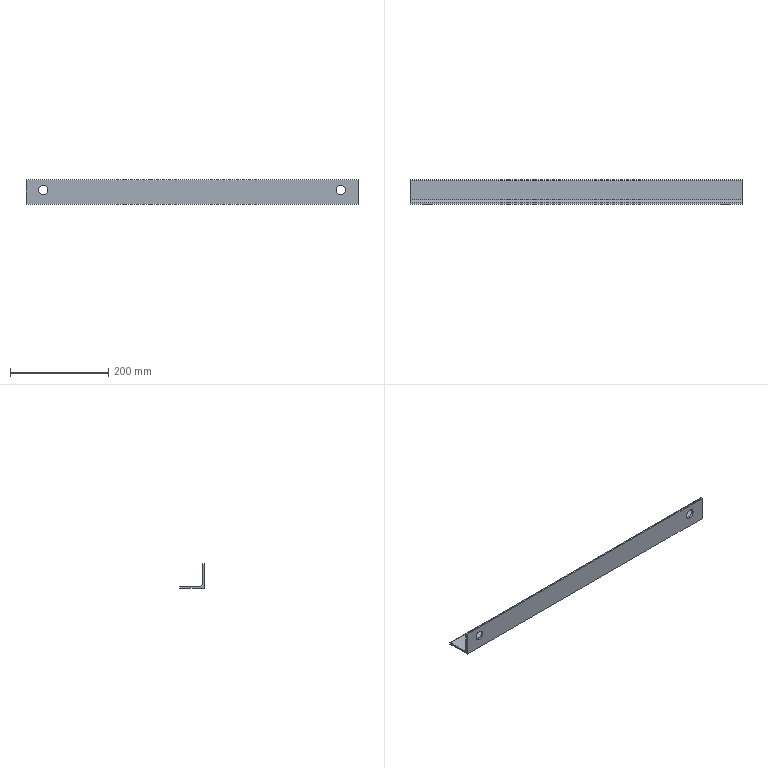Part | STEP file | 电柜角钢2_Default<As Machined> | 1 solid | 15 faces | box 675 x 50 x 50 mm | volume 260801 mm3 | plane 8 | cylinder 7 | commonest cylinder face diameters 19 x4 2.66 x2 11 x1
STEP:
#1=CARTESIAN_POINT('',(0.,0.,0.));
#2=DIRECTION('',(0.,0.,1.));
#3=DIRECTION('',(1.,0.,0.));
#4=AXIS2_PLACEMENT_3D('',#1,#2,#3);
#5=CARTESIAN_POINT('',(-302.5,0.,38.585));
#6=VERTEX_POINT('',#5);
#7=CARTESIAN_POINT('',(-302.5,4.,38.585));
#8=VERTEX_POINT('',#7);
#9=CARTESIAN_POINT('',(-302.5,-6.,38.585));
#10=DIRECTION('',(0.,1.,0.));
#11=VECTOR('',#10,1.);
#12=LINE('',#9,#11);
#13=CARTESIAN_POINT('',(-302.5,-6.,29.085));
#14=DIRECTION('',(0.,1.,0.));
#15=DIRECTION('',(0.,0.,1.));
#16=AXIS2_PLACEMENT_3D('',#13,#14,#15);
#17=CYLINDRICAL_SURFACE('',#16,9.5);
#18=CARTESIAN_POINT('',(6.283,0.));
#19=DIRECTION('',(0.,1.));
#20=VECTOR('',#19,1.);
#21=LINE('',#18,#20);
#22=(GEOMETRIC_REPRESENTATION_CONTEXT(2)PARAMETRIC_REPRESENTATION_CONTEXT()REPRESENTATION_CONTEXT('',''));
#23=DEFINITIONAL_REPRESENTATION('',(#21),#22);
#24=PCURVE('',#17,#23);
#25=CARTESIAN_POINT('',(-302.5,-6.,29.085));
#26=DIRECTION('',(0.,1.,0.));
#27=DIRECTION('',(0.,0.,1.));
#28=AXIS2_PLACEMENT_3D('',#25,#26,#27);
#29=CYLINDRICAL_SURFACE('',#28,9.5);
#30=CARTESIAN_POINT('',(0.,0.));
#31=DIRECTION('',(0.,1.));
#32=VECTOR('',#31,1.);
#33=LINE('',#30,#32);
#34=(GEOMETRIC_REPRESENTATION_CONTEXT(2)PARAMETRIC_REPRESENTATION_CONTEXT()REPRESENTATION_CONTEXT('',''));
#35=DEFINITIONAL_REPRESENTATION('',(#33),#34);
#36=PCURVE('',#29,#35);
#37=SURFACE_CURVE('',#12,(#24,#36),.PCURVE_S1.);
#38=EDGE_CURVE('',#6,#8,#37,.T.);
#39=ORIENTED_EDGE('',*,*,#38,.T.);
#40=CARTESIAN_POINT('',(-302.5,4.,19.585));
#41=VERTEX_POINT('',#40);
#42=CARTESIAN_POINT('',(-302.5,4.,29.085));
#43=DIRECTION('',(0.,1.,0.));
#44=DIRECTION('',(0.,0.,1.));
#45=AXIS2_PLACEMENT_3D('',#42,#43,#44);
#46=CIRCLE('',#45,9.5);
#47=CARTESIAN_POINT('',(0.,10.));
#48=DIRECTION('',(1.,0.));
#49=VECTOR('',#48,1.);
#50=LINE('',#47,#49);
#51=(GEOMETRIC_REPRESENTATION_CONTEXT(2)PARAMETRIC_REPRESENTATION_CONTEXT()REPRESENTATION_CONTEXT('',''));
#52=DEFINITIONAL_REPRESENTATION('',(#50),#51);
#53=PCURVE('',#17,#52);
#54=CARTESIAN_POINT('',(337.5,4.,48.67));
#55=DIRECTION('',(0.,-1.,0.));
#56=DIRECTION('',(1.,0.,0.));
#57=AXIS2_PLACEMENT_3D('',#54,#55,#56);
#58=PLANE('',#57);
#59=CARTESIAN_POINT('',(-640.,-10.085));
#60=CARTESIAN_POINT('',(-623.546,-10.085));
#61=CARTESIAN_POINT('',(-631.773,-24.335));
#62=CARTESIAN_POINT('',(-640.,-38.585));
#63=CARTESIAN_POINT('',(-648.227,-24.335));
#64=CARTESIAN_POINT('',(-656.454,-10.085));
#65=CARTESIAN_POINT('',(-640.,-10.085));
#66=(BOUNDED_CURVE()B_SPLINE_CURVE(2,(#59,#60,#61,#62,#63,#64,#65),.UNSPECIFIED.,.T.,.F.)B_SPLINE_CURVE_WITH_KNOTS((1,2,2,2,2,1),(-2.094,0.,2.094,4.189,6.283,8.378),.UNSPECIFIED.)CURVE()GEOMETRIC_REPRESENTATION_ITEM()RATIONAL_B_SPLINE_CURVE((1.,0.5,1.,0.5,1.,0.5,1.))REPRESENTATION_ITEM(''));
#67=(GEOMETRIC_REPRESENTATION_CONTEXT(2)PARAMETRIC_REPRESENTATION_CONTEXT()REPRESENTATION_CONTEXT('',''));
#68=DEFINITIONAL_REPRESENTATION('',(#66),#67);
#69=PCURVE('',#58,#68);
#70=SURFACE_CURVE('',#46,(#53,#69),.PCURVE_S1.);
#71=EDGE_CURVE('',#41,#8,#70,.T.);
#72=ORIENTED_EDGE('',*,*,#71,.F.);
#73=CARTESIAN_POINT('',(-302.5,0.,19.585));
#74=VERTEX_POINT('',#73);
#75=CARTESIAN_POINT('',(-302.5,-6.,19.585));
#76=DIRECTION('',(0.,1.,0.));
#77=VECTOR('',#76,1.);
#78=LINE('',#75,#77);
#79=CARTESIAN_POINT('',(3.142,0.));
#80=DIRECTION('',(0.,1.));
#81=VECTOR('',#80,1.);
#82=LINE('',#79,#81);
#83=(GEOMETRIC_REPRESENTATION_CONTEXT(2)PARAMETRIC_REPRESENTATION_CONTEXT()REPRESENTATION_CONTEXT('',''));
#84=DEFINITIONAL_REPRESENTATION('',(#82),#83);
#85=PCURVE('',#17,#84);
#86=CARTESIAN_POINT('',(3.142,0.));
#87=DIRECTION('',(0.,1.));
#88=VECTOR('',#87,1.);
#89=LINE('',#86,#88);
#90=(GEOMETRIC_REPRESENTATION_CONTEXT(2)PARAMETRIC_REPRESENTATION_CONTEXT()REPRESENTATION_CONTEXT('',''));
#91=DEFINITIONAL_REPRESENTATION('',(#89),#90);
#92=PCURVE('',#29,#91);
#93=SURFACE_CURVE('',#78,(#85,#92),.PCURVE_S1.);
#94=EDGE_CURVE('',#74,#41,#93,.T.);
#95=ORIENTED_EDGE('',*,*,#94,.F.);
#96=CARTESIAN_POINT('',(-302.5,0.,29.085));
#97=DIRECTION('',(0.,1.,0.));
#98=DIRECTION('',(-1.,0.,0.));
#99=AXIS2_PLACEMENT_3D('',#96,#97,#98);
#100=CIRCLE('',#99,9.5);
#101=CARTESIAN_POINT('',(-1.571,6.));
#102=DIRECTION('',(1.,0.));
#103=VECTOR('',#102,1.);
#104=LINE('',#101,#103);
#105=(GEOMETRIC_REPRESENTATION_CONTEXT(2)PARAMETRIC_REPRESENTATION_CONTEXT()REPRESENTATION_CONTEXT('',''));
#106=DEFINITIONAL_REPRESENTATION('',(#104),#105);
#107=PCURVE('',#17,#106);
#108=CARTESIAN_POINT('',(337.5,0.,50.));
#109=DIRECTION('',(0.,1.,0.));
#110=DIRECTION('',(-1.,0.,0.));
#111=AXIS2_PLACEMENT_3D('',#108,#109,#110);
#112=PLANE('',#111);
#113=CARTESIAN_POINT('',(640.,-20.915));
#114=DIRECTION('',(1.,0.));
#115=AXIS2_PLACEMENT_2D('',#113,#114);
#116=CIRCLE('',#115,9.5);
#117=(GEOMETRIC_REPRESENTATION_CONTEXT(2)PARAMETRIC_REPRESENTATION_CONTEXT()REPRESENTATION_CONTEXT('',''));
#118=DEFINITIONAL_REPRESENTATION('',(#116),#117);
#119=PCURVE('',#112,#118);
#120=SURFACE_CURVE('',#100,(#107,#119),.PCURVE_S1.);
#121=EDGE_CURVE('',#74,#6,#120,.T.);
#122=ORIENTED_EDGE('',*,*,#121,.T.);
#123=EDGE_LOOP('',(#39,#72,#95,#122));
#124=FACE_BOUND('',#123,.F.);
#125=ADVANCED_FACE('',(#124),#17,.F.);
#126=CARTESIAN_POINT('',(302.5,0.,38.585));
#127=VERTEX_POINT('',#126);
#128=CARTESIAN_POINT('',(302.5,4.,38.585));
#129=VERTEX_POINT('',#128);
#130=CARTESIAN_POINT('',(302.5,-6.,38.585));
#131=DIRECTION('',(0.,1.,0.));
#132=VECTOR('',#131,1.);
#133=LINE('',#130,#132);
#134=CARTESIAN_POINT('',(302.5,-6.,29.085));
#135=DIRECTION('',(0.,1.,0.));
#136=DIRECTION('',(0.,0.,1.));
#137=AXIS2_PLACEMENT_3D('',#134,#135,#136);
#138=CYLINDRICAL_SURFACE('',#137,9.5);
#139=CARTESIAN_POINT('',(6.283,0.));
#140=DIRECTION('',(0.,1.));
#141=VECTOR('',#140,1.);
#142=LINE('',#139,#141);
#143=(GEOMETRIC_REPRESENTATION_CONTEXT(2)PARAMETRIC_REPRESENTATION_CONTEXT()REPRESENTATION_CONTEXT('',''));
#144=DEFINITIONAL_REPRESENTATION('',(#142),#143);
#145=PCURVE('',#138,#144);
#146=CARTESIAN_POINT('',(302.5,-6.,29.085));
#147=DIRECTION('',(0.,1.,0.));
#148=DIRECTION('',(0.,0.,1.));
#149=AXIS2_PLACEMENT_3D('',#146,#147,#148);
#150=CYLINDRICAL_SURFACE('',#149,9.5);
#151=CARTESIAN_POINT('',(0.,0.));
#152=DIRECTION('',(0.,1.));
#153=VECTOR('',#152,1.);
#154=LINE('',#151,#153);
#155=(GEOMETRIC_REPRESENTATION_CONTEXT(2)PARAMETRIC_REPRESENTATION_CONTEXT()REPRESENTATION_CONTEXT('',''));
#156=DEFINITIONAL_REPRESENTATION('',(#154),#155);
#157=PCURVE('',#150,#156);
#158=SURFACE_CURVE('',#133,(#145,#157),.PCURVE_S1.);
#159=EDGE_CURVE('',#127,#129,#158,.T.);
#160=ORIENTED_EDGE('',*,*,#159,.T.);
#161=CARTESIAN_POINT('',(302.5,4.,19.585));
#162=VERTEX_POINT('',#161);
#163=CARTESIAN_POINT('',(302.5,4.,29.085));
#164=DIRECTION('',(0.,1.,0.));
#165=DIRECTION('',(0.,0.,-1.));
#166=AXIS2_PLACEMENT_3D('',#163,#164,#165);
#167=CIRCLE('',#166,9.5);
#168=CARTESIAN_POINT('',(3.142,10.));
#169=DIRECTION('',(1.,0.));
#170=VECTOR('',#169,1.);
#171=LINE('',#168,#170);
#172=(GEOMETRIC_REPRESENTATION_CONTEXT(2)PARAMETRIC_REPRESENTATION_CONTEXT()REPRESENTATION_CONTEXT('',''));
#173=DEFINITIONAL_REPRESENTATION('',(#171),#172);
#174=PCURVE('',#138,#173);
#175=CARTESIAN_POINT('',(-35.,-29.085));
#176=CARTESIAN_POINT('',(-51.454,-29.085));
#177=CARTESIAN_POINT('',(-43.227,-14.835));
#178=CARTESIAN_POINT('',(-35.,-0.585));
#179=CARTESIAN_POINT('',(-26.773,-14.835));
#180=CARTESIAN_POINT('',(-18.546,-29.085));
#181=CARTESIAN_POINT('',(-35.,-29.085));
#182=(BOUNDED_CURVE()B_SPLINE_CURVE(2,(#175,#176,#177,#178,#179,#180,#181),.UNSPECIFIED.,.T.,.F.)B_SPLINE_CURVE_WITH_KNOTS((1,2,2,2,2,1),(-2.094,0.,2.094,4.189,6.283,8.378),.UNSPECIFIED.)CURVE()GEOMETRIC_REPRESENTATION_ITEM()RATIONAL_B_SPLINE_CURVE((1.,0.5,1.,0.5,1.,0.5,1.))REPRESENTATION_ITEM(''));
#183=(GEOMETRIC_REPRESENTATION_CONTEXT(2)PARAMETRIC_REPRESENTATION_CONTEXT()REPRESENTATION_CONTEXT('',''));
#184=DEFINITIONAL_REPRESENTATION('',(#182),#183);
#185=PCURVE('',#58,#184);
#186=SURFACE_CURVE('',#167,(#174,#185),.PCURVE_S1.);
#187=EDGE_CURVE('',#162,#129,#186,.T.);
#188=ORIENTED_EDGE('',*,*,#187,.F.);
#189=CARTESIAN_POINT('',(302.5,0.,19.585));
#190=VERTEX_POINT('',#189);
#191=CARTESIAN_POINT('',(302.5,-6.,19.585));
#192=DIRECTION('',(0.,1.,0.));
#193=VECTOR('',#192,1.);
#194=LINE('',#191,#193);
#195=CARTESIAN_POINT('',(3.142,0.));
#196=DIRECTION('',(0.,1.));
#197=VECTOR('',#196,1.);
#198=LINE('',#195,#197);
#199=(GEOMETRIC_REPRESENTATION_CONTEXT(2)PARAMETRIC_REPRESENTATION_CONTEXT()REPRESENTATION_CONTEXT('',''));
#200=DEFINITIONAL_REPRESENTATION('',(#198),#199);
#201=PCURVE('',#138,#200);
#202=CARTESIAN_POINT('',(3.142,0.));
#203=DIRECTION('',(0.,1.));
#204=VECTOR('',#203,1.);
#205=LINE('',#202,#204);
#206=(GEOMETRIC_REPRESENTATION_CONTEXT(2)PARAMETRIC_REPRESENTATION_CONTEXT()REPRESENTATION_CONTEXT('',''));
#207=DEFINITIONAL_REPRESENTATION('',(#205),#206);
#208=PCURVE('',#150,#207);
#209=SURFACE_CURVE('',#194,(#201,#208),.PCURVE_S1.);
#210=EDGE_CURVE('',#190,#162,#209,.T.);
#211=ORIENTED_EDGE('',*,*,#210,.F.);
#212=CARTESIAN_POINT('',(302.5,0.,29.085));
#213=DIRECTION('',(0.,1.,0.));
#214=DIRECTION('',(-1.,0.,0.));
#215=AXIS2_PLACEMENT_3D('',#212,#213,#214);
#216=CIRCLE('',#215,9.5);
#217=CARTESIAN_POINT('',(-1.571,6.));
#218=DIRECTION('',(1.,0.));
#219=VECTOR('',#218,1.);
#220=LINE('',#217,#219);
#221=(GEOMETRIC_REPRESENTATION_CONTEXT(2)PARAMETRIC_REPRESENTATION_CONTEXT()REPRESENTATION_CONTEXT('',''));
#222=DEFINITIONAL_REPRESENTATION('',(#220),#221);
#223=PCURVE('',#138,#222);
#224=CARTESIAN_POINT('',(35.,-20.915));
#225=DIRECTION('',(1.,0.));
#226=AXIS2_PLACEMENT_2D('',#224,#225);
#227=CIRCLE('',#226,9.5);
#228=(GEOMETRIC_REPRESENTATION_CONTEXT(2)PARAMETRIC_REPRESENTATION_CONTEXT()REPRESENTATION_CONTEXT('',''));
#229=DEFINITIONAL_REPRESENTATION('',(#227),#228);
#230=PCURVE('',#112,#229);
#231=SURFACE_CURVE('',#216,(#223,#230),.PCURVE_S1.);
#232=EDGE_CURVE('',#190,#127,#231,.T.);
#233=ORIENTED_EDGE('',*,*,#232,.T.);
#234=EDGE_LOOP('',(#160,#188,#211,#233));
#235=FACE_BOUND('',#234,.F.);
#236=ADVANCED_FACE('',(#235),#138,.F.);
#237=CARTESIAN_POINT('',(-337.5,50.,2.67));
#238=VERTEX_POINT('',#237);
#239=CARTESIAN_POINT('',(-337.5,48.67,4.));
#240=VERTEX_POINT('',#239);
#241=CARTESIAN_POINT('',(-337.5,48.67,2.67));
#242=DIRECTION('',(1.,0.,0.));
#243=DIRECTION('',(0.,1.,0.));
#244=AXIS2_PLACEMENT_3D('',#241,#242,#243);
#245=CIRCLE('',#244,1.33);
#246=CARTESIAN_POINT('',(337.5,48.67,2.67));
#247=DIRECTION('',(-1.,0.,0.));
#248=DIRECTION('',(0.,-1.,0.));
#249=AXIS2_PLACEMENT_3D('',#246,#247,#248);
#250=CYLINDRICAL_SURFACE('',#249,1.33);
#251=CARTESIAN_POINT('',(3.142,675.));
#252=DIRECTION('',(-1.,0.));
#253=VECTOR('',#252,1.);
#254=LINE('',#251,#253);
#255=(GEOMETRIC_REPRESENTATION_CONTEXT(2)PARAMETRIC_REPRESENTATION_CONTEXT()REPRESENTATION_CONTEXT('',''));
#256=DEFINITIONAL_REPRESENTATION('',(#254),#255);
#257=PCURVE('',#250,#256);
#258=CARTESIAN_POINT('',(-337.5,48.67,2.67));
#259=DIRECTION('',(1.,0.,0.));
#260=DIRECTION('',(0.,1.,0.));
#261=AXIS2_PLACEMENT_3D('',#258,#259,#260);
#262=PLANE('',#261);
#263=CARTESIAN_POINT('',(0.,0.));
#264=DIRECTION('',(1.,0.));
#265=AXIS2_PLACEMENT_2D('',#263,#264);
#266=CIRCLE('',#265,1.33);
#267=(GEOMETRIC_REPRESENTATION_CONTEXT(2)PARAMETRIC_REPRESENTATION_CONTEXT()REPRESENTATION_CONTEXT('',''));
#268=DEFINITIONAL_REPRESENTATION('',(#266),#267);
#269=PCURVE('',#262,#268);
#270=SURFACE_CURVE('',#245,(#257,#269),.PCURVE_S1.);
#271=EDGE_CURVE('',#238,#240,#270,.T.);
#272=ORIENTED_EDGE('',*,*,#271,.T.);
#273=CARTESIAN_POINT('',(337.5,48.67,4.));
#274=VERTEX_POINT('',#273);
#275=CARTESIAN_POINT('',(337.5,48.67,4.));
#276=DIRECTION('',(-1.,0.,0.));
#277=VECTOR('',#276,1.);
#278=LINE('',#275,#277);
#279=CARTESIAN_POINT('',(1.571,0.));
#280=DIRECTION('',(0.,1.));
#281=VECTOR('',#280,1.);
#282=LINE('',#279,#281);
#283=(GEOMETRIC_REPRESENTATION_CONTEXT(2)PARAMETRIC_REPRESENTATION_CONTEXT()REPRESENTATION_CONTEXT('',''));
#284=DEFINITIONAL_REPRESENTATION('',(#282),#283);
#285=PCURVE('',#250,#284);
#286=CARTESIAN_POINT('',(337.5,9.5,4.));
#287=DIRECTION('',(0.,0.,-1.));
#288=DIRECTION('',(-1.,0.,0.));
#289=AXIS2_PLACEMENT_3D('',#286,#287,#288);
#290=PLANE('',#289);
#291=CARTESIAN_POINT('',(0.,39.17));
#292=DIRECTION('',(1.,0.));
#293=VECTOR('',#292,1.);
#294=LINE('',#291,#293);
#295=(GEOMETRIC_REPRESENTATION_CONTEXT(2)PARAMETRIC_REPRESENTATION_CONTEXT()REPRESENTATION_CONTEXT('',''));
#296=DEFINITIONAL_REPRESENTATION('',(#294),#295);
#297=PCURVE('',#290,#296);
#298=SURFACE_CURVE('',#278,(#285,#297),.PCURVE_S1.);
#299=EDGE_CURVE('',#274,#240,#298,.T.);
#300=ORIENTED_EDGE('',*,*,#299,.F.);
#301=CARTESIAN_POINT('',(337.5,50.,2.67));
#302=VERTEX_POINT('',#301);
#303=CARTESIAN_POINT('',(337.5,48.67,2.67));
#304=DIRECTION('',(1.,0.,0.));
#305=DIRECTION('',(0.,1.,0.));
#306=AXIS2_PLACEMENT_3D('',#303,#304,#305);
#307=CIRCLE('',#306,1.33);
#308=CARTESIAN_POINT('',(3.142,0.));
#309=DIRECTION('',(-1.,0.));
#310=VECTOR('',#309,1.);
#311=LINE('',#308,#310);
#312=(GEOMETRIC_REPRESENTATION_CONTEXT(2)PARAMETRIC_REPRESENTATION_CONTEXT()REPRESENTATION_CONTEXT('',''));
#313=DEFINITIONAL_REPRESENTATION('',(#311),#312);
#314=PCURVE('',#250,#313);
#315=CARTESIAN_POINT('',(337.5,48.67,2.67));
#316=DIRECTION('',(1.,0.,0.));
#317=DIRECTION('',(0.,1.,0.));
#318=AXIS2_PLACEMENT_3D('',#315,#316,#317);
#319=PLANE('',#318);
#320=CARTESIAN_POINT('',(0.,0.));
#321=DIRECTION('',(1.,0.));
#322=AXIS2_PLACEMENT_2D('',#320,#321);
#323=CIRCLE('',#322,1.33);
#324=(GEOMETRIC_REPRESENTATION_CONTEXT(2)PARAMETRIC_REPRESENTATION_CONTEXT()REPRESENTATION_CONTEXT('',''));
#325=DEFINITIONAL_REPRESENTATION('',(#323),#324);
#326=PCURVE('',#319,#325);
#327=SURFACE_CURVE('',#307,(#314,#326),.PCURVE_S1.);
#328=EDGE_CURVE('',#302,#274,#327,.T.);
#329=ORIENTED_EDGE('',*,*,#328,.F.);
#330=CARTESIAN_POINT('',(337.5,50.,2.67));
#331=DIRECTION('',(-1.,0.,0.));
#332=VECTOR('',#331,1.);
#333=LINE('',#330,#332);
#334=CARTESIAN_POINT('',(3.142,0.));
#335=DIRECTION('',(0.,1.));
#336=VECTOR('',#335,1.);
#337=LINE('',#334,#336);
#338=(GEOMETRIC_REPRESENTATION_CONTEXT(2)PARAMETRIC_REPRESENTATION_CONTEXT()REPRESENTATION_CONTEXT('',''));
#339=DEFINITIONAL_REPRESENTATION('',(#337),#338);
#340=PCURVE('',#250,#339);
#341=CARTESIAN_POINT('',(337.5,50.,2.67));
#342=DIRECTION('',(0.,-1.,0.));
#343=DIRECTION('',(1.,0.,0.));
#344=AXIS2_PLACEMENT_3D('',#341,#342,#343);
#345=PLANE('',#344);
#346=CARTESIAN_POINT('',(0.,0.));
#347=DIRECTION('',(-1.,0.));
#348=VECTOR('',#347,1.);
#349=LINE('',#346,#348);
#350=(GEOMETRIC_REPRESENTATION_CONTEXT(2)PARAMETRIC_REPRESENTATION_CONTEXT()REPRESENTATION_CONTEXT('',''));
#351=DEFINITIONAL_REPRESENTATION('',(#349),#350);
#352=PCURVE('',#345,#351);
#353=SURFACE_CURVE('',#333,(#340,#352),.PCURVE_S1.);
#354=EDGE_CURVE('',#302,#238,#353,.T.);
#355=ORIENTED_EDGE('',*,*,#354,.T.);
#356=EDGE_LOOP('',(#272,#300,#329,#355));
#357=FACE_BOUND('',#356,.T.);
#358=ADVANCED_FACE('',(#357),#250,.T.);
#359=CARTESIAN_POINT('',(-337.5,9.5,4.));
#360=VERTEX_POINT('',#359);
#361=CARTESIAN_POINT('',(-337.5,9.5,4.));
#362=DIRECTION('',(0.,-1.,0.));
#363=VECTOR('',#362,1.);
#364=LINE('',#361,#363);
#365=CARTESIAN_POINT('',(675.,0.));
#366=DIRECTION('',(0.,-1.));
#367=VECTOR('',#366,1.);
#368=LINE('',#365,#367);
#369=(GEOMETRIC_REPRESENTATION_CONTEXT(2)PARAMETRIC_REPRESENTATION_CONTEXT()REPRESENTATION_CONTEXT('',''));
#370=DEFINITIONAL_REPRESENTATION('',(#368),#369);
#371=PCURVE('',#290,#370);
#372=CARTESIAN_POINT('',(-39.17,1.33));
#373=DIRECTION('',(-1.,0.));
#374=VECTOR('',#373,1.);
#375=LINE('',#372,#374);
#376=(GEOMETRIC_REPRESENTATION_CONTEXT(2)PARAMETRIC_REPRESENTATION_CONTEXT()REPRESENTATION_CONTEXT('',''));
#377=DEFINITIONAL_REPRESENTATION('',(#375),#376);
#378=PCURVE('',#262,#377);
#379=SURFACE_CURVE('',#364,(#371,#378),.PCURVE_S1.);
#380=EDGE_CURVE('',#240,#360,#379,.T.);
#381=ORIENTED_EDGE('',*,*,#380,.T.);
#382=CARTESIAN_POINT('',(337.5,9.5,4.));
#383=VERTEX_POINT('',#382);
#384=CARTESIAN_POINT('',(337.5,9.5,4.));
#385=DIRECTION('',(-1.,0.,0.));
#386=VECTOR('',#385,1.);
#387=LINE('',#384,#386);
#388=CARTESIAN_POINT('',(0.,0.));
#389=DIRECTION('',(1.,0.));
#390=VECTOR('',#389,1.);
#391=LINE('',#388,#390);
#392=(GEOMETRIC_REPRESENTATION_CONTEXT(2)PARAMETRIC_REPRESENTATION_CONTEXT()REPRESENTATION_CONTEXT('',''));
#393=DEFINITIONAL_REPRESENTATION('',(#391),#392);
#394=PCURVE('',#290,#393);
#395=CARTESIAN_POINT('',(337.5,9.5,9.5));
#396=DIRECTION('',(-1.,0.,0.));
#397=DIRECTION('',(0.,-1.,0.));
#398=AXIS2_PLACEMENT_3D('',#395,#396,#397);
#399=CYLINDRICAL_SURFACE('',#398,5.5);
#400=CARTESIAN_POINT('',(4.712,0.));
#401=DIRECTION('',(0.,1.));
#402=VECTOR('',#401,1.);
#403=LINE('',#400,#402);
#404=(GEOMETRIC_REPRESENTATION_CONTEXT(2)PARAMETRIC_REPRESENTATION_CONTEXT()REPRESENTATION_CONTEXT('',''));
#405=DEFINITIONAL_REPRESENTATION('',(#403),#404);
#406=PCURVE('',#399,#405);
#407=SURFACE_CURVE('',#387,(#394,#406),.PCURVE_S1.);
#408=EDGE_CURVE('',#383,#360,#407,.T.);
#409=ORIENTED_EDGE('',*,*,#408,.F.);
#410=CARTESIAN_POINT('',(337.5,9.5,4.));
#411=DIRECTION('',(0.,-1.,0.));
#412=VECTOR('',#411,1.);
#413=LINE('',#410,#412);
#414=CARTESIAN_POINT('',(0.,0.));
#415=DIRECTION('',(0.,-1.));
#416=VECTOR('',#415,1.);
#417=LINE('',#414,#416);
#418=(GEOMETRIC_REPRESENTATION_CONTEXT(2)PARAMETRIC_REPRESENTATION_CONTEXT()REPRESENTATION_CONTEXT('',''));
#419=DEFINITIONAL_REPRESENTATION('',(#417),#418);
#420=PCURVE('',#290,#419);
#421=CARTESIAN_POINT('',(-39.17,1.33));
#422=DIRECTION('',(-1.,0.));
#423=VECTOR('',#422,1.);
#424=LINE('',#421,#423);
#425=(GEOMETRIC_REPRESENTATION_CONTEXT(2)PARAMETRIC_REPRESENTATION_CONTEXT()REPRESENTATION_CONTEXT('',''));
#426=DEFINITIONAL_REPRESENTATION('',(#424),#425);
#427=PCURVE('',#319,#426);
#428=SURFACE_CURVE('',#413,(#420,#427),.PCURVE_S1.);
#429=EDGE_CURVE('',#274,#383,#428,.T.);
#430=ORIENTED_EDGE('',*,*,#429,.F.);
#431=ORIENTED_EDGE('',*,*,#299,.T.);
#432=EDGE_LOOP('',(#381,#409,#430,#431));
#433=FACE_BOUND('',#432,.T.);
#434=ADVANCED_FACE('',(#433),#290,.F.);
#435=ORIENTED_EDGE('',*,*,#408,.F.);
#436=CARTESIAN_POINT('',(337.5,4.,9.5));
#437=VERTEX_POINT('',#436);
#438=CARTESIAN_POINT('',(337.5,9.5,9.5));
#439=DIRECTION('',(-1.,0.,0.));
#440=DIRECTION('',(0.,1.,0.));
#441=AXIS2_PLACEMENT_3D('',#438,#439,#440);
#442=CIRCLE('',#441,5.5);
#443=CARTESIAN_POINT('',(3.142,0.));
#444=DIRECTION('',(1.,0.));
#445=VECTOR('',#444,1.);
#446=LINE('',#443,#445);
#447=(GEOMETRIC_REPRESENTATION_CONTEXT(2)PARAMETRIC_REPRESENTATION_CONTEXT()REPRESENTATION_CONTEXT('',''));
#448=DEFINITIONAL_REPRESENTATION('',(#446),#447);
#449=PCURVE('',#399,#448);
#450=CARTESIAN_POINT('',(-33.67,6.83));
#451=CARTESIAN_POINT('',(-33.67,-2.696));
#452=CARTESIAN_POINT('',(-41.92,2.067));
#453=CARTESIAN_POINT('',(-50.17,6.83));
#454=CARTESIAN_POINT('',(-41.92,11.593));
#455=CARTESIAN_POINT('',(-33.67,16.356));
#456=CARTESIAN_POINT('',(-33.67,6.83));
#457=(BOUNDED_CURVE()B_SPLINE_CURVE(2,(#450,#451,#452,#453,#454,#455,#456),.UNSPECIFIED.,.T.,.F.)B_SPLINE_CURVE_WITH_KNOTS((1,2,2,2,2,1),(-2.094,0.,2.094,4.189,6.283,8.378),.UNSPECIFIED.)CURVE()GEOMETRIC_REPRESENTATION_ITEM()RATIONAL_B_SPLINE_CURVE((1.,0.5,1.,0.5,1.,0.5,1.))REPRESENTATION_ITEM(''));
#458=(GEOMETRIC_REPRESENTATION_CONTEXT(2)PARAMETRIC_REPRESENTATION_CONTEXT()REPRESENTATION_CONTEXT('',''));
#459=DEFINITIONAL_REPRESENTATION('',(#457),#458);
#460=PCURVE('',#319,#459);
#461=SURFACE_CURVE('',#442,(#449,#460),.PCURVE_S1.);
#462=EDGE_CURVE('',#383,#437,#461,.T.);
#463=ORIENTED_EDGE('',*,*,#462,.T.);
#464=CARTESIAN_POINT('',(-337.5,4.,9.5));
#465=VERTEX_POINT('',#464);
#466=CARTESIAN_POINT('',(337.5,4.,9.5));
#467=DIRECTION('',(-1.,0.,0.));
#468=VECTOR('',#467,1.);
#469=LINE('',#466,#468);
#470=CARTESIAN_POINT('',(6.283,0.));
#471=DIRECTION('',(0.,1.));
#472=VECTOR('',#471,1.);
#473=LINE('',#470,#472);
#474=(GEOMETRIC_REPRESENTATION_CONTEXT(2)PARAMETRIC_REPRESENTATION_CONTEXT()REPRESENTATION_CONTEXT('',''));
#475=DEFINITIONAL_REPRESENTATION('',(#473),#474);
#476=PCURVE('',#399,#475);
#477=CARTESIAN_POINT('',(0.,-39.17));
#478=DIRECTION('',(-1.,0.));
#479=VECTOR('',#478,1.);
#480=LINE('',#477,#479);
#481=(GEOMETRIC_REPRESENTATION_CONTEXT(2)PARAMETRIC_REPRESENTATION_CONTEXT()REPRESENTATION_CONTEXT('',''));
#482=DEFINITIONAL_REPRESENTATION('',(#480),#481);
#483=PCURVE('',#58,#482);
#484=SURFACE_CURVE('',#469,(#476,#483),.PCURVE_S1.);
#485=EDGE_CURVE('',#437,#465,#484,.T.);
#486=ORIENTED_EDGE('',*,*,#485,.T.);
#487=CARTESIAN_POINT('',(-337.5,9.5,9.5));
#488=DIRECTION('',(-1.,0.,0.));
#489=DIRECTION('',(0.,1.,0.));
#490=AXIS2_PLACEMENT_3D('',#487,#488,#489);
#491=CIRCLE('',#490,5.5);
#492=CARTESIAN_POINT('',(3.142,675.));
#493=DIRECTION('',(1.,0.));
#494=VECTOR('',#493,1.);
#495=LINE('',#492,#494);
#496=(GEOMETRIC_REPRESENTATION_CONTEXT(2)PARAMETRIC_REPRESENTATION_CONTEXT()REPRESENTATION_CONTEXT('',''));
#497=DEFINITIONAL_REPRESENTATION('',(#495),#496);
#498=PCURVE('',#399,#497);
#499=CARTESIAN_POINT('',(-33.67,6.83));
#500=CARTESIAN_POINT('',(-33.67,-2.696));
#501=CARTESIAN_POINT('',(-41.92,2.067));
#502=CARTESIAN_POINT('',(-50.17,6.83));
#503=CARTESIAN_POINT('',(-41.92,11.593));
#504=CARTESIAN_POINT('',(-33.67,16.356));
#505=CARTESIAN_POINT('',(-33.67,6.83));
#506=(BOUNDED_CURVE()B_SPLINE_CURVE(2,(#499,#500,#501,#502,#503,#504,#505),.UNSPECIFIED.,.T.,.F.)B_SPLINE_CURVE_WITH_KNOTS((1,2,2,2,2,1),(-2.094,0.,2.094,4.189,6.283,8.378),.UNSPECIFIED.)CURVE()GEOMETRIC_REPRESENTATION_ITEM()RATIONAL_B_SPLINE_CURVE((1.,0.5,1.,0.5,1.,0.5,1.))REPRESENTATION_ITEM(''));
#507=(GEOMETRIC_REPRESENTATION_CONTEXT(2)PARAMETRIC_REPRESENTATION_CONTEXT()REPRESENTATION_CONTEXT('',''));
#508=DEFINITIONAL_REPRESENTATION('',(#506),#507);
#509=PCURVE('',#262,#508);
#510=SURFACE_CURVE('',#491,(#498,#509),.PCURVE_S1.);
#511=EDGE_CURVE('',#360,#465,#510,.T.);
#512=ORIENTED_EDGE('',*,*,#511,.F.);
#513=EDGE_LOOP('',(#435,#463,#486,#512));
#514=FACE_BOUND('',#513,.F.);
#515=ADVANCED_FACE('',(#514),#399,.F.);
#516=CARTESIAN_POINT('',(-302.5,4.,29.085));
#517=DIRECTION('',(0.,1.,0.));
#518=DIRECTION('',(0.,0.,1.));
#519=AXIS2_PLACEMENT_3D('',#516,#517,#518);
#520=CIRCLE('',#519,9.5);
#521=CARTESIAN_POINT('',(-640.,-10.085));
#522=CARTESIAN_POINT('',(-623.546,-10.085));
#523=CARTESIAN_POINT('',(-631.773,-24.335));
#524=CARTESIAN_POINT('',(-640.,-38.585));
#525=CARTESIAN_POINT('',(-648.227,-24.335));
#526=CARTESIAN_POINT('',(-656.454,-10.085));
#527=CARTESIAN_POINT('',(-640.,-10.085));
#528=(BOUNDED_CURVE()B_SPLINE_CURVE(2,(#521,#522,#523,#524,#525,#526,#527),.UNSPECIFIED.,.T.,.F.)B_SPLINE_CURVE_WITH_KNOTS((1,2,2,2,2,1),(-2.094,0.,2.094,4.189,6.283,8.378),.UNSPECIFIED.)CURVE()GEOMETRIC_REPRESENTATION_ITEM()RATIONAL_B_SPLINE_CURVE((1.,0.5,1.,0.5,1.,0.5,1.))REPRESENTATION_ITEM(''));
#529=(GEOMETRIC_REPRESENTATION_CONTEXT(2)PARAMETRIC_REPRESENTATION_CONTEXT()REPRESENTATION_CONTEXT('',''));
#530=DEFINITIONAL_REPRESENTATION('',(#528),#529);
#531=PCURVE('',#58,#530);
#532=CARTESIAN_POINT('',(0.,10.));
#533=DIRECTION('',(1.,0.));
#534=VECTOR('',#533,1.);
#535=LINE('',#532,#534);
#536=(GEOMETRIC_REPRESENTATION_CONTEXT(2)PARAMETRIC_REPRESENTATION_CONTEXT()REPRESENTATION_CONTEXT('',''));
#537=DEFINITIONAL_REPRESENTATION('',(#535),#536);
#538=PCURVE('',#29,#537);
#539=SURFACE_CURVE('',#520,(#531,#538),.PCURVE_S1.);
#540=EDGE_CURVE('',#8,#41,#539,.T.);
#541=ORIENTED_EDGE('',*,*,#540,.F.);
#542=ORIENTED_EDGE('',*,*,#71,.F.);
#543=EDGE_LOOP('',(#541,#542));
#544=FACE_BOUND('',#543,.T.);
#545=CARTESIAN_POINT('',(302.5,4.,29.085));
#546=DIRECTION('',(0.,1.,0.));
#547=DIRECTION('',(0.,0.,-1.));
#548=AXIS2_PLACEMENT_3D('',#545,#546,#547);
#549=CIRCLE('',#548,9.5);
#550=CARTESIAN_POINT('',(-35.,-29.085));
#551=CARTESIAN_POINT('',(-51.454,-29.085));
#552=CARTESIAN_POINT('',(-43.227,-14.835));
#553=CARTESIAN_POINT('',(-35.,-0.585));
#554=CARTESIAN_POINT('',(-26.773,-14.835));
#555=CARTESIAN_POINT('',(-18.546,-29.085));
#556=CARTESIAN_POINT('',(-35.,-29.085));
#557=(BOUNDED_CURVE()B_SPLINE_CURVE(2,(#550,#551,#552,#553,#554,#555,#556),.UNSPECIFIED.,.T.,.F.)B_SPLINE_CURVE_WITH_KNOTS((1,2,2,2,2,1),(-2.094,0.,2.094,4.189,6.283,8.378),.UNSPECIFIED.)CURVE()GEOMETRIC_REPRESENTATION_ITEM()RATIONAL_B_SPLINE_CURVE((1.,0.5,1.,0.5,1.,0.5,1.))REPRESENTATION_ITEM(''));
#558=(GEOMETRIC_REPRESENTATION_CONTEXT(2)PARAMETRIC_REPRESENTATION_CONTEXT()REPRESENTATION_CONTEXT('',''));
#559=DEFINITIONAL_REPRESENTATION('',(#557),#558);
#560=PCURVE('',#58,#559);
#561=CARTESIAN_POINT('',(-3.142,10.));
#562=DIRECTION('',(1.,0.));
#563=VECTOR('',#562,1.);
#564=LINE('',#561,#563);
#565=(GEOMETRIC_REPRESENTATION_CONTEXT(2)PARAMETRIC_REPRESENTATION_CONTEXT()REPRESENTATION_CONTEXT('',''));
#566=DEFINITIONAL_REPRESENTATION('',(#564),#565);
#567=PCURVE('',#150,#566);
#568=SURFACE_CURVE('',#549,(#560,#567),.PCURVE_S1.);
#569=EDGE_CURVE('',#129,#162,#568,.T.);
#570=ORIENTED_EDGE('',*,*,#569,.F.);
#571=ORIENTED_EDGE('',*,*,#187,.F.);
#572=EDGE_LOOP('',(#570,#571));
#573=FACE_BOUND('',#572,.T.);
#574=CARTESIAN_POINT('',(-337.5,4.,48.67));
#575=VERTEX_POINT('',#574);
#576=CARTESIAN_POINT('',(-337.5,4.,48.67));
#577=DIRECTION('',(0.,0.,1.));
#578=VECTOR('',#577,1.);
#579=LINE('',#576,#578);
#580=CARTESIAN_POINT('',(-675.,0.));
#581=DIRECTION('',(0.,1.));
#582=VECTOR('',#581,1.);
#583=LINE('',#580,#582);
#584=(GEOMETRIC_REPRESENTATION_CONTEXT(2)PARAMETRIC_REPRESENTATION_CONTEXT()REPRESENTATION_CONTEXT('',''));
#585=DEFINITIONAL_REPRESENTATION('',(#583),#584);
#586=PCURVE('',#58,#585);
#587=CARTESIAN_POINT('',(-44.67,46.));
#588=DIRECTION('',(0.,1.));
#589=VECTOR('',#588,1.);
#590=LINE('',#587,#589);
#591=(GEOMETRIC_REPRESENTATION_CONTEXT(2)PARAMETRIC_REPRESENTATION_CONTEXT()REPRESENTATION_CONTEXT('',''));
#592=DEFINITIONAL_REPRESENTATION('',(#590),#591);
#593=PCURVE('',#262,#592);
#594=SURFACE_CURVE('',#579,(#586,#593),.PCURVE_S1.);
#595=EDGE_CURVE('',#465,#575,#594,.T.);
#596=ORIENTED_EDGE('',*,*,#595,.T.);
#597=CARTESIAN_POINT('',(337.5,4.,48.67));
#598=VERTEX_POINT('',#597);
#599=CARTESIAN_POINT('',(337.5,4.,48.67));
#600=DIRECTION('',(-1.,0.,0.));
#601=VECTOR('',#600,1.);
#602=LINE('',#599,#601);
#603=CARTESIAN_POINT('',(0.,0.));
#604=DIRECTION('',(-1.,0.));
#605=VECTOR('',#604,1.);
#606=LINE('',#603,#605);
#607=(GEOMETRIC_REPRESENTATION_CONTEXT(2)PARAMETRIC_REPRESENTATION_CONTEXT()REPRESENTATION_CONTEXT('',''));
#608=DEFINITIONAL_REPRESENTATION('',(#606),#607);
#609=PCURVE('',#58,#608);
#610=CARTESIAN_POINT('',(337.5,2.67,48.67));
#611=DIRECTION('',(-1.,0.,0.));
#612=DIRECTION('',(0.,-1.,0.));
#613=AXIS2_PLACEMENT_3D('',#610,#611,#612);
#614=CYLINDRICAL_SURFACE('',#613,1.33);
#615=CARTESIAN_POINT('',(3.142,0.));
#616=DIRECTION('',(0.,1.));
#617=VECTOR('',#616,1.);
#618=LINE('',#615,#617);
#619=(GEOMETRIC_REPRESENTATION_CONTEXT(2)PARAMETRIC_REPRESENTATION_CONTEXT()REPRESENTATION_CONTEXT('',''));
#620=DEFINITIONAL_REPRESENTATION('',(#618),#619);
#621=PCURVE('',#614,#620);
#622=SURFACE_CURVE('',#602,(#609,#621),.PCURVE_S1.);
#623=EDGE_CURVE('',#598,#575,#622,.T.);
#624=ORIENTED_EDGE('',*,*,#623,.F.);
#625=CARTESIAN_POINT('',(337.5,4.,48.67));
#626=DIRECTION('',(0.,0.,1.));
#627=VECTOR('',#626,1.);
#628=LINE('',#625,#627);
#629=CARTESIAN_POINT('',(0.,0.));
#630=DIRECTION('',(0.,1.));
#631=VECTOR('',#630,1.);
#632=LINE('',#629,#631);
#633=(GEOMETRIC_REPRESENTATION_CONTEXT(2)PARAMETRIC_REPRESENTATION_CONTEXT()REPRESENTATION_CONTEXT('',''));
#634=DEFINITIONAL_REPRESENTATION('',(#632),#633);
#635=PCURVE('',#58,#634);
#636=CARTESIAN_POINT('',(-44.67,46.));
#637=DIRECTION('',(0.,1.));
#638=VECTOR('',#637,1.);
#639=LINE('',#636,#638);
#640=(GEOMETRIC_REPRESENTATION_CONTEXT(2)PARAMETRIC_REPRESENTATION_CONTEXT()REPRESENTATION_CONTEXT('',''));
#641=DEFINITIONAL_REPRESENTATION('',(#639),#640);
#642=PCURVE('',#319,#641);
#643=SURFACE_CURVE('',#628,(#635,#642),.PCURVE_S1.);
#644=EDGE_CURVE('',#437,#598,#643,.T.);
#645=ORIENTED_EDGE('',*,*,#644,.F.);
#646=ORIENTED_EDGE('',*,*,#485,.T.);
#647=EDGE_LOOP('',(#596,#624,#645,#646));
#648=FACE_BOUND('',#647,.T.);
#649=ADVANCED_FACE('',(#544,#573,#648),#58,.F.);
#650=CARTESIAN_POINT('',(-337.5,2.67,50.));
#651=VERTEX_POINT('',#650);
#652=CARTESIAN_POINT('',(-337.5,2.67,48.67));
#653=DIRECTION('',(1.,0.,0.));
#654=DIRECTION('',(0.,1.,0.));
#655=AXIS2_PLACEMENT_3D('',#652,#653,#654);
#656=CIRCLE('',#655,1.33);
#657=CARTESIAN_POINT('',(3.142,675.));
#658=DIRECTION('',(-1.,0.));
#659=VECTOR('',#658,1.);
#660=LINE('',#657,#659);
#661=(GEOMETRIC_REPRESENTATION_CONTEXT(2)PARAMETRIC_REPRESENTATION_CONTEXT()REPRESENTATION_CONTEXT('',''));
#662=DEFINITIONAL_REPRESENTATION('',(#660),#661);
#663=PCURVE('',#614,#662);
#664=CARTESIAN_POINT('',(-46.,46.));
#665=DIRECTION('',(1.,0.));
#666=AXIS2_PLACEMENT_2D('',#664,#665);
#667=CIRCLE('',#666,1.33);
#668=(GEOMETRIC_REPRESENTATION_CONTEXT(2)PARAMETRIC_REPRESENTATION_CONTEXT()REPRESENTATION_CONTEXT('',''));
#669=DEFINITIONAL_REPRESENTATION('',(#667),#668);
#670=PCURVE('',#262,#669);
#671=SURFACE_CURVE('',#656,(#663,#670),.PCURVE_S1.);
#672=EDGE_CURVE('',#575,#651,#671,.T.);
#673=ORIENTED_EDGE('',*,*,#672,.T.);
#674=CARTESIAN_POINT('',(337.5,2.67,50.));
#675=VERTEX_POINT('',#674);
#676=CARTESIAN_POINT('',(337.5,2.67,50.));
#677=DIRECTION('',(-1.,0.,0.));
#678=VECTOR('',#677,1.);
#679=LINE('',#676,#678);
#680=CARTESIAN_POINT('',(1.571,0.));
#681=DIRECTION('',(0.,1.));
#682=VECTOR('',#681,1.);
#683=LINE('',#680,#682);
#684=(GEOMETRIC_REPRESENTATION_CONTEXT(2)PARAMETRIC_REPRESENTATION_CONTEXT()REPRESENTATION_CONTEXT('',''));
#685=DEFINITIONAL_REPRESENTATION('',(#683),#684);
#686=PCURVE('',#614,#685);
#687=CARTESIAN_POINT('',(337.5,0.,50.));
#688=DIRECTION('',(0.,0.,-1.));
#689=DIRECTION('',(0.,1.,0.));
#690=AXIS2_PLACEMENT_3D('',#687,#688,#689);
#691=PLANE('',#690);
#692=CARTESIAN_POINT('',(2.67,0.));
#693=DIRECTION('',(0.,-1.));
#694=VECTOR('',#693,1.);
#695=LINE('',#692,#694);
#696=(GEOMETRIC_REPRESENTATION_CONTEXT(2)PARAMETRIC_REPRESENTATION_CONTEXT()REPRESENTATION_CONTEXT('',''));
#697=DEFINITIONAL_REPRESENTATION('',(#695),#696);
#698=PCURVE('',#691,#697);
#699=SURFACE_CURVE('',#679,(#686,#698),.PCURVE_S1.);
#700=EDGE_CURVE('',#675,#651,#699,.T.);
#701=ORIENTED_EDGE('',*,*,#700,.F.);
#702=CARTESIAN_POINT('',(337.5,2.67,48.67));
#703=DIRECTION('',(1.,0.,0.));
#704=DIRECTION('',(0.,1.,0.));
#705=AXIS2_PLACEMENT_3D('',#702,#703,#704);
#706=CIRCLE('',#705,1.33);
#707=CARTESIAN_POINT('',(3.142,0.));
#708=DIRECTION('',(-1.,0.));
#709=VECTOR('',#708,1.);
#710=LINE('',#707,#709);
#711=(GEOMETRIC_REPRESENTATION_CONTEXT(2)PARAMETRIC_REPRESENTATION_CONTEXT()REPRESENTATION_CONTEXT('',''));
#712=DEFINITIONAL_REPRESENTATION('',(#710),#711);
#713=PCURVE('',#614,#712);
#714=CARTESIAN_POINT('',(-46.,46.));
#715=DIRECTION('',(1.,0.));
#716=AXIS2_PLACEMENT_2D('',#714,#715);
#717=CIRCLE('',#716,1.33);
#718=(GEOMETRIC_REPRESENTATION_CONTEXT(2)PARAMETRIC_REPRESENTATION_CONTEXT()REPRESENTATION_CONTEXT('',''));
#719=DEFINITIONAL_REPRESENTATION('',(#717),#718);
#720=PCURVE('',#319,#719);
#721=SURFACE_CURVE('',#706,(#713,#720),.PCURVE_S1.);
#722=EDGE_CURVE('',#598,#675,#721,.T.);
#723=ORIENTED_EDGE('',*,*,#722,.F.);
#724=ORIENTED_EDGE('',*,*,#623,.T.);
#725=EDGE_LOOP('',(#673,#701,#723,#724));
#726=FACE_BOUND('',#725,.T.);
#727=ADVANCED_FACE('',(#726),#614,.T.);
#728=CARTESIAN_POINT('',(-337.5,0.,50.));
#729=VERTEX_POINT('',#728);
#730=CARTESIAN_POINT('',(-337.5,0.,50.));
#731=DIRECTION('',(0.,-1.,0.));
#732=VECTOR('',#731,1.);
#733=LINE('',#730,#732);
#734=CARTESIAN_POINT('',(0.,-675.));
#735=DIRECTION('',(-1.,0.));
#736=VECTOR('',#735,1.);
#737=LINE('',#734,#736);
#738=(GEOMETRIC_REPRESENTATION_CONTEXT(2)PARAMETRIC_REPRESENTATION_CONTEXT()REPRESENTATION_CONTEXT('',''));
#739=DEFINITIONAL_REPRESENTATION('',(#737),#738);
#740=PCURVE('',#691,#739);
#741=CARTESIAN_POINT('',(-48.67,47.33));
#742=DIRECTION('',(-1.,0.));
#743=VECTOR('',#742,1.);
#744=LINE('',#741,#743);
#745=(GEOMETRIC_REPRESENTATION_CONTEXT(2)PARAMETRIC_REPRESENTATION_CONTEXT()REPRESENTATION_CONTEXT('',''));
#746=DEFINITIONAL_REPRESENTATION('',(#744),#745);
#747=PCURVE('',#262,#746);
#748=SURFACE_CURVE('',#733,(#740,#747),.PCURVE_S1.);
#749=EDGE_CURVE('',#651,#729,#748,.T.);
#750=ORIENTED_EDGE('',*,*,#749,.T.);
#751=CARTESIAN_POINT('',(337.5,0.,50.));
#752=VERTEX_POINT('',#751);
#753=CARTESIAN_POINT('',(337.5,0.,50.));
#754=DIRECTION('',(-1.,0.,0.));
#755=VECTOR('',#754,1.);
#756=LINE('',#753,#755);
#757=CARTESIAN_POINT('',(0.,0.));
#758=DIRECTION('',(0.,-1.));
#759=VECTOR('',#758,1.);
#760=LINE('',#757,#759);
#761=(GEOMETRIC_REPRESENTATION_CONTEXT(2)PARAMETRIC_REPRESENTATION_CONTEXT()REPRESENTATION_CONTEXT('',''));
#762=DEFINITIONAL_REPRESENTATION('',(#760),#761);
#763=PCURVE('',#691,#762);
#764=CARTESIAN_POINT('',(0.,0.));
#765=DIRECTION('',(1.,0.));
#766=VECTOR('',#765,1.);
#767=LINE('',#764,#766);
#768=(GEOMETRIC_REPRESENTATION_CONTEXT(2)PARAMETRIC_REPRESENTATION_CONTEXT()REPRESENTATION_CONTEXT('',''));
#769=DEFINITIONAL_REPRESENTATION('',(#767),#768);
#770=PCURVE('',#112,#769);
#771=SURFACE_CURVE('',#756,(#763,#770),.PCURVE_S1.);
#772=EDGE_CURVE('',#752,#729,#771,.T.);
#773=ORIENTED_EDGE('',*,*,#772,.F.);
#774=CARTESIAN_POINT('',(337.5,0.,50.));
#775=DIRECTION('',(0.,-1.,0.));
#776=VECTOR('',#775,1.);
#777=LINE('',#774,#776);
#778=CARTESIAN_POINT('',(0.,0.));
#779=DIRECTION('',(-1.,0.));
#780=VECTOR('',#779,1.);
#781=LINE('',#778,#780);
#782=(GEOMETRIC_REPRESENTATION_CONTEXT(2)PARAMETRIC_REPRESENTATION_CONTEXT()REPRESENTATION_CONTEXT('',''));
#783=DEFINITIONAL_REPRESENTATION('',(#781),#782);
#784=PCURVE('',#691,#783);
#785=CARTESIAN_POINT('',(-48.67,47.33));
#786=DIRECTION('',(-1.,0.));
#787=VECTOR('',#786,1.);
#788=LINE('',#785,#787);
#789=(GEOMETRIC_REPRESENTATION_CONTEXT(2)PARAMETRIC_REPRESENTATION_CONTEXT()REPRESENTATION_CONTEXT('',''));
#790=DEFINITIONAL_REPRESENTATION('',(#788),#789);
#791=PCURVE('',#319,#790);
#792=SURFACE_CURVE('',#777,(#784,#791),.PCURVE_S1.);
#793=EDGE_CURVE('',#675,#752,#792,.T.);
#794=ORIENTED_EDGE('',*,*,#793,.F.);
#795=ORIENTED_EDGE('',*,*,#700,.T.);
#796=EDGE_LOOP('',(#750,#773,#794,#795));
#797=FACE_BOUND('',#796,.T.);
#798=ADVANCED_FACE('',(#797),#691,.F.);
#799=CARTESIAN_POINT('',(-302.5,0.,29.085));
#800=DIRECTION('',(0.,1.,0.));
#801=DIRECTION('',(-1.,0.,0.));
#802=AXIS2_PLACEMENT_3D('',#799,#800,#801);
#803=CIRCLE('',#802,9.5);
#804=CARTESIAN_POINT('',(640.,-20.915));
#805=DIRECTION('',(1.,0.));
#806=AXIS2_PLACEMENT_2D('',#804,#805);
#807=CIRCLE('',#806,9.5);
#808=(GEOMETRIC_REPRESENTATION_CONTEXT(2)PARAMETRIC_REPRESENTATION_CONTEXT()REPRESENTATION_CONTEXT('',''));
#809=DEFINITIONAL_REPRESENTATION('',(#807),#808);
#810=PCURVE('',#112,#809);
#811=CARTESIAN_POINT('',(-1.571,6.));
#812=DIRECTION('',(1.,0.));
#813=VECTOR('',#812,1.);
#814=LINE('',#811,#813);
#815=(GEOMETRIC_REPRESENTATION_CONTEXT(2)PARAMETRIC_REPRESENTATION_CONTEXT()REPRESENTATION_CONTEXT('',''));
#816=DEFINITIONAL_REPRESENTATION('',(#814),#815);
#817=PCURVE('',#29,#816);
#818=SURFACE_CURVE('',#803,(#810,#817),.PCURVE_S1.);
#819=EDGE_CURVE('',#6,#74,#818,.T.);
#820=ORIENTED_EDGE('',*,*,#819,.T.);
#821=ORIENTED_EDGE('',*,*,#121,.T.);
#822=EDGE_LOOP('',(#820,#821));
#823=FACE_BOUND('',#822,.T.);
#824=CARTESIAN_POINT('',(302.5,0.,29.085));
#825=DIRECTION('',(0.,1.,0.));
#826=DIRECTION('',(-1.,0.,0.));
#827=AXIS2_PLACEMENT_3D('',#824,#825,#826);
#828=CIRCLE('',#827,9.5);
#829=CARTESIAN_POINT('',(35.,-20.915));
#830=DIRECTION('',(1.,0.));
#831=AXIS2_PLACEMENT_2D('',#829,#830);
#832=CIRCLE('',#831,9.5);
#833=(GEOMETRIC_REPRESENTATION_CONTEXT(2)PARAMETRIC_REPRESENTATION_CONTEXT()REPRESENTATION_CONTEXT('',''));
#834=DEFINITIONAL_REPRESENTATION('',(#832),#833);
#835=PCURVE('',#112,#834);
#836=CARTESIAN_POINT('',(-1.571,6.));
#837=DIRECTION('',(1.,0.));
#838=VECTOR('',#837,1.);
#839=LINE('',#836,#838);
#840=(GEOMETRIC_REPRESENTATION_CONTEXT(2)PARAMETRIC_REPRESENTATION_CONTEXT()REPRESENTATION_CONTEXT('',''));
#841=DEFINITIONAL_REPRESENTATION('',(#839),#840);
#842=PCURVE('',#150,#841);
#843=SURFACE_CURVE('',#828,(#835,#842),.PCURVE_S1.);
#844=EDGE_CURVE('',#127,#190,#843,.T.);
#845=ORIENTED_EDGE('',*,*,#844,.T.);
#846=ORIENTED_EDGE('',*,*,#232,.T.);
#847=EDGE_LOOP('',(#845,#846));
#848=FACE_BOUND('',#847,.T.);
#849=CARTESIAN_POINT('',(-337.5,0.,0.));
#850=VERTEX_POINT('',#849);
#851=CARTESIAN_POINT('',(-337.5,0.,50.));
#852=DIRECTION('',(0.,0.,-1.));
#853=VECTOR('',#852,1.);
#854=LINE('',#851,#853);
#855=CARTESIAN_POINT('',(675.,0.));
#856=DIRECTION('',(0.,-1.));
#857=VECTOR('',#856,1.);
#858=LINE('',#855,#857);
#859=(GEOMETRIC_REPRESENTATION_CONTEXT(2)PARAMETRIC_REPRESENTATION_CONTEXT()REPRESENTATION_CONTEXT('',''));
#860=DEFINITIONAL_REPRESENTATION('',(#858),#859);
#861=PCURVE('',#112,#860);
#862=CARTESIAN_POINT('',(-48.67,47.33));
#863=DIRECTION('',(0.,-1.));
#864=VECTOR('',#863,1.);
#865=LINE('',#862,#864);
#866=(GEOMETRIC_REPRESENTATION_CONTEXT(2)PARAMETRIC_REPRESENTATION_CONTEXT()REPRESENTATION_CONTEXT('',''));
#867=DEFINITIONAL_REPRESENTATION('',(#865),#866);
#868=PCURVE('',#262,#867);
#869=SURFACE_CURVE('',#854,(#861,#868),.PCURVE_S1.);
#870=EDGE_CURVE('',#729,#850,#869,.T.);
#871=ORIENTED_EDGE('',*,*,#870,.T.);
#872=CARTESIAN_POINT('',(337.5,0.,0.));
#873=VERTEX_POINT('',#872);
#874=CARTESIAN_POINT('',(337.5,0.,0.));
#875=DIRECTION('',(-1.,0.,0.));
#876=VECTOR('',#875,1.);
#877=LINE('',#874,#876);
#878=CARTESIAN_POINT('',(0.,-50.));
#879=DIRECTION('',(1.,0.));
#880=VECTOR('',#879,1.);
#881=LINE('',#878,#880);
#882=(GEOMETRIC_REPRESENTATION_CONTEXT(2)PARAMETRIC_REPRESENTATION_CONTEXT()REPRESENTATION_CONTEXT('',''));
#883=DEFINITIONAL_REPRESENTATION('',(#881),#882);
#884=PCURVE('',#112,#883);
#885=CARTESIAN_POINT('',(337.5,0.,0.));
#886=DIRECTION('',(0.,0.,1.));
#887=DIRECTION('',(1.,0.,0.));
#888=AXIS2_PLACEMENT_3D('',#885,#886,#887);
#889=PLANE('',#888);
#890=CARTESIAN_POINT('',(0.,0.));
#891=DIRECTION('',(-1.,0.));
#892=VECTOR('',#891,1.);
#893=LINE('',#890,#892);
#894=(GEOMETRIC_REPRESENTATION_CONTEXT(2)PARAMETRIC_REPRESENTATION_CONTEXT()REPRESENTATION_CONTEXT('',''));
#895=DEFINITIONAL_REPRESENTATION('',(#893),#894);
#896=PCURVE('',#889,#895);
#897=SURFACE_CURVE('',#877,(#884,#896),.PCURVE_S1.);
#898=EDGE_CURVE('',#873,#850,#897,.T.);
#899=ORIENTED_EDGE('',*,*,#898,.F.);
#900=CARTESIAN_POINT('',(337.5,0.,50.));
#901=DIRECTION('',(0.,0.,-1.));
#902=VECTOR('',#901,1.);
#903=LINE('',#900,#902);
#904=CARTESIAN_POINT('',(0.,0.));
#905=DIRECTION('',(0.,-1.));
#906=VECTOR('',#905,1.);
#907=LINE('',#904,#906);
#908=(GEOMETRIC_REPRESENTATION_CONTEXT(2)PARAMETRIC_REPRESENTATION_CONTEXT()REPRESENTATION_CONTEXT('',''));
#909=DEFINITIONAL_REPRESENTATION('',(#907),#908);
#910=PCURVE('',#112,#909);
#911=CARTESIAN_POINT('',(-48.67,47.33));
#912=DIRECTION('',(0.,-1.));
#913=VECTOR('',#912,1.);
#914=LINE('',#911,#913);
#915=(GEOMETRIC_REPRESENTATION_CONTEXT(2)PARAMETRIC_REPRESENTATION_CONTEXT()REPRESENTATION_CONTEXT('',''));
#916=DEFINITIONAL_REPRESENTATION('',(#914),#915);
#917=PCURVE('',#319,#916);
#918=SURFACE_CURVE('',#903,(#910,#917),.PCURVE_S1.);
#919=EDGE_CURVE('',#752,#873,#918,.T.);
#920=ORIENTED_EDGE('',*,*,#919,.F.);
#921=ORIENTED_EDGE('',*,*,#772,.T.);
#922=EDGE_LOOP('',(#871,#899,#920,#921));
#923=FACE_BOUND('',#922,.T.);
#924=ADVANCED_FACE('',(#823,#848,#923),#112,.F.);
#925=CARTESIAN_POINT('',(-337.5,50.,0.));
#926=VERTEX_POINT('',#925);
#927=CARTESIAN_POINT('',(-337.5,0.,0.));
#928=DIRECTION('',(0.,1.,0.));
#929=VECTOR('',#928,1.);
#930=LINE('',#927,#929);
#931=CARTESIAN_POINT('',(-675.,0.));
#932=DIRECTION('',(0.,1.));
#933=VECTOR('',#932,1.);
#934=LINE('',#931,#933);
#935=(GEOMETRIC_REPRESENTATION_CONTEXT(2)PARAMETRIC_REPRESENTATION_CONTEXT()REPRESENTATION_CONTEXT('',''));
#936=DEFINITIONAL_REPRESENTATION('',(#934),#935);
#937=PCURVE('',#889,#936);
#938=CARTESIAN_POINT('',(-48.67,-2.67));
#939=DIRECTION('',(1.,0.));
#940=VECTOR('',#939,1.);
#941=LINE('',#938,#940);
#942=(GEOMETRIC_REPRESENTATION_CONTEXT(2)PARAMETRIC_REPRESENTATION_CONTEXT()REPRESENTATION_CONTEXT('',''));
#943=DEFINITIONAL_REPRESENTATION('',(#941),#942);
#944=PCURVE('',#262,#943);
#945=SURFACE_CURVE('',#930,(#937,#944),.PCURVE_S1.);
#946=EDGE_CURVE('',#850,#926,#945,.T.);
#947=ORIENTED_EDGE('',*,*,#946,.T.);
#948=CARTESIAN_POINT('',(337.5,50.,0.));
#949=VERTEX_POINT('',#948);
#950=CARTESIAN_POINT('',(337.5,50.,0.));
#951=DIRECTION('',(-1.,0.,0.));
#952=VECTOR('',#951,1.);
#953=LINE('',#950,#952);
#954=CARTESIAN_POINT('',(0.,50.));
#955=DIRECTION('',(-1.,0.));
#956=VECTOR('',#955,1.);
#957=LINE('',#954,#956);
#958=(GEOMETRIC_REPRESENTATION_CONTEXT(2)PARAMETRIC_REPRESENTATION_CONTEXT()REPRESENTATION_CONTEXT('',''));
#959=DEFINITIONAL_REPRESENTATION('',(#957),#958);
#960=PCURVE('',#889,#959);
#961=CARTESIAN_POINT('',(0.,-2.67));
#962=DIRECTION('',(-1.,0.));
#963=VECTOR('',#962,1.);
#964=LINE('',#961,#963);
#965=(GEOMETRIC_REPRESENTATION_CONTEXT(2)PARAMETRIC_REPRESENTATION_CONTEXT()REPRESENTATION_CONTEXT('',''));
#966=DEFINITIONAL_REPRESENTATION('',(#964),#965);
#967=PCURVE('',#345,#966);
#968=SURFACE_CURVE('',#953,(#960,#967),.PCURVE_S1.);
#969=EDGE_CURVE('',#949,#926,#968,.T.);
#970=ORIENTED_EDGE('',*,*,#969,.F.);
#971=CARTESIAN_POINT('',(337.5,0.,0.));
#972=DIRECTION('',(0.,1.,0.));
#973=VECTOR('',#972,1.);
#974=LINE('',#971,#973);
#975=CARTESIAN_POINT('',(0.,0.));
#976=DIRECTION('',(0.,1.));
#977=VECTOR('',#976,1.);
#978=LINE('',#975,#977);
#979=(GEOMETRIC_REPRESENTATION_CONTEXT(2)PARAMETRIC_REPRESENTATION_CONTEXT()REPRESENTATION_CONTEXT('',''));
#980=DEFINITIONAL_REPRESENTATION('',(#978),#979);
#981=PCURVE('',#889,#980);
#982=CARTESIAN_POINT('',(-48.67,-2.67));
#983=DIRECTION('',(1.,0.));
#984=VECTOR('',#983,1.);
#985=LINE('',#982,#984);
#986=(GEOMETRIC_REPRESENTATION_CONTEXT(2)PARAMETRIC_REPRESENTATION_CONTEXT()REPRESENTATION_CONTEXT('',''));
#987=DEFINITIONAL_REPRESENTATION('',(#985),#986);
#988=PCURVE('',#319,#987);
#989=SURFACE_CURVE('',#974,(#981,#988),.PCURVE_S1.);
#990=EDGE_CURVE('',#873,#949,#989,.T.);
#991=ORIENTED_EDGE('',*,*,#990,.F.);
#992=ORIENTED_EDGE('',*,*,#898,.T.);
#993=EDGE_LOOP('',(#947,#970,#991,#992));
#994=FACE_BOUND('',#993,.T.);
#995=ADVANCED_FACE('',(#994),#889,.F.);
#996=CARTESIAN_POINT('',(-337.5,50.,2.67));
#997=DIRECTION('',(0.,0.,1.));
#998=VECTOR('',#997,1.);
#999=LINE('',#996,#998);
#1000=CARTESIAN_POINT('',(-675.,0.));
#1001=DIRECTION('',(0.,1.));
#1002=VECTOR('',#1001,1.);
#1003=LINE('',#1000,#1002);
#1004=(GEOMETRIC_REPRESENTATION_CONTEXT(2)PARAMETRIC_REPRESENTATION_CONTEXT()REPRESENTATION_CONTEXT('',''));
#1005=DEFINITIONAL_REPRESENTATION('',(#1003),#1004);
#1006=PCURVE('',#345,#1005);
#1007=CARTESIAN_POINT('',(1.33,0.));
#1008=DIRECTION('',(0.,1.));
#1009=VECTOR('',#1008,1.);
#1010=LINE('',#1007,#1009);
#1011=(GEOMETRIC_REPRESENTATION_CONTEXT(2)PARAMETRIC_REPRESENTATION_CONTEXT()REPRESENTATION_CONTEXT('',''));
#1012=DEFINITIONAL_REPRESENTATION('',(#1010),#1011);
#1013=PCURVE('',#262,#1012);
#1014=SURFACE_CURVE('',#999,(#1006,#1013),.PCURVE_S1.);
#1015=EDGE_CURVE('',#926,#238,#1014,.T.);
#1016=ORIENTED_EDGE('',*,*,#1015,.T.);
#1017=ORIENTED_EDGE('',*,*,#354,.F.);
#1018=CARTESIAN_POINT('',(337.5,50.,2.67));
#1019=DIRECTION('',(0.,0.,1.));
#1020=VECTOR('',#1019,1.);
#1021=LINE('',#1018,#1020);
#1022=CARTESIAN_POINT('',(0.,0.));
#1023=DIRECTION('',(0.,1.));
#1024=VECTOR('',#1023,1.);
#1025=LINE('',#1022,#1024);
#1026=(GEOMETRIC_REPRESENTATION_CONTEXT(2)PARAMETRIC_REPRESENTATION_CONTEXT()REPRESENTATION_CONTEXT('',''));
#1027=DEFINITIONAL_REPRESENTATION('',(#1025),#1026);
#1028=PCURVE('',#345,#1027);
#1029=CARTESIAN_POINT('',(1.33,0.));
#1030=DIRECTION('',(0.,1.));
#1031=VECTOR('',#1030,1.);
#1032=LINE('',#1029,#1031);
#1033=(GEOMETRIC_REPRESENTATION_CONTEXT(2)PARAMETRIC_REPRESENTATION_CONTEXT()REPRESENTATION_CONTEXT('',''));
#1034=DEFINITIONAL_REPRESENTATION('',(#1032),#1033);
#1035=PCURVE('',#319,#1034);
#1036=SURFACE_CURVE('',#1021,(#1028,#1035),.PCURVE_S1.);
#1037=EDGE_CURVE('',#949,#302,#1036,.T.);
#1038=ORIENTED_EDGE('',*,*,#1037,.F.);
#1039=ORIENTED_EDGE('',*,*,#969,.T.);
#1040=EDGE_LOOP('',(#1016,#1017,#1038,#1039));
#1041=FACE_BOUND('',#1040,.T.);
#1042=ADVANCED_FACE('',(#1041),#345,.F.);
#1043=ORIENTED_EDGE('',*,*,#328,.T.);
#1044=ORIENTED_EDGE('',*,*,#429,.T.);
#1045=ORIENTED_EDGE('',*,*,#462,.T.);
#1046=ORIENTED_EDGE('',*,*,#644,.T.);
#1047=ORIENTED_EDGE('',*,*,#722,.T.);
#1048=ORIENTED_EDGE('',*,*,#793,.T.);
#1049=ORIENTED_EDGE('',*,*,#919,.T.);
#1050=ORIENTED_EDGE('',*,*,#990,.T.);
#1051=ORIENTED_EDGE('',*,*,#1037,.T.);
#1052=EDGE_LOOP('',(#1043,#1044,#1045,#1046,#1047,#1048,#1049,#1050,#1051));
#1053=FACE_BOUND('',#1052,.T.);
#1054=ADVANCED_FACE('',(#1053),#319,.T.);
#1055=ORIENTED_EDGE('',*,*,#271,.F.);
#1056=ORIENTED_EDGE('',*,*,#1015,.F.);
#1057=ORIENTED_EDGE('',*,*,#946,.F.);
#1058=ORIENTED_EDGE('',*,*,#870,.F.);
#1059=ORIENTED_EDGE('',*,*,#749,.F.);
#1060=ORIENTED_EDGE('',*,*,#672,.F.);
#1061=ORIENTED_EDGE('',*,*,#595,.F.);
#1062=ORIENTED_EDGE('',*,*,#511,.F.);
#1063=ORIENTED_EDGE('',*,*,#380,.F.);
#1064=EDGE_LOOP('',(#1055,#1056,#1057,#1058,#1059,#1060,#1061,#1062,#1063));
#1065=FACE_BOUND('',#1064,.T.);
#1066=ADVANCED_FACE('',(#1065),#262,.F.);
#1067=ORIENTED_EDGE('',*,*,#569,.F.);
#1068=ORIENTED_EDGE('',*,*,#159,.F.);
#1069=ORIENTED_EDGE('',*,*,#844,.T.);
#1070=ORIENTED_EDGE('',*,*,#210,.T.);
#1071=EDGE_LOOP('',(#1067,#1068,#1069,#1070));
#1072=FACE_BOUND('',#1071,.F.);
#1073=ADVANCED_FACE('',(#1072),#150,.F.);
#1074=ORIENTED_EDGE('',*,*,#540,.F.);
#1075=ORIENTED_EDGE('',*,*,#38,.F.);
#1076=ORIENTED_EDGE('',*,*,#819,.T.);
#1077=ORIENTED_EDGE('',*,*,#94,.T.);
#1078=EDGE_LOOP('',(#1074,#1075,#1076,#1077));
#1079=FACE_BOUND('',#1078,.F.);
#1080=ADVANCED_FACE('',(#1079),#29,.F.);
#1081=CLOSED_SHELL('',(#125,#236,#358,#434,#515,#649,#727,#798,#924,#995,#1042,#1054,#1066,#1073,#1080));
#1082=MANIFOLD_SOLID_BREP('',#1081);
#1083=(LENGTH_UNIT()NAMED_UNIT(*)SI_UNIT(.MILLI.,.METRE.));
#1084=UNCERTAINTY_MEASURE_WITH_UNIT(LENGTH_MEASURE(0.0000001),#1083,'','');
#1085=(NAMED_UNIT(*)PLANE_ANGLE_UNIT()SI_UNIT($,.RADIAN.));
#1086=(NAMED_UNIT(*)SI_UNIT($,.STERADIAN.)SOLID_ANGLE_UNIT());
#1087=(GEOMETRIC_REPRESENTATION_CONTEXT(3)GLOBAL_UNCERTAINTY_ASSIGNED_CONTEXT((#1084))GLOBAL_UNIT_ASSIGNED_CONTEXT((#1083,#1085,#1086))REPRESENTATION_CONTEXT('',''));
#1088=ADVANCED_BREP_SHAPE_REPRESENTATION('',(#4,#1082),#1087);